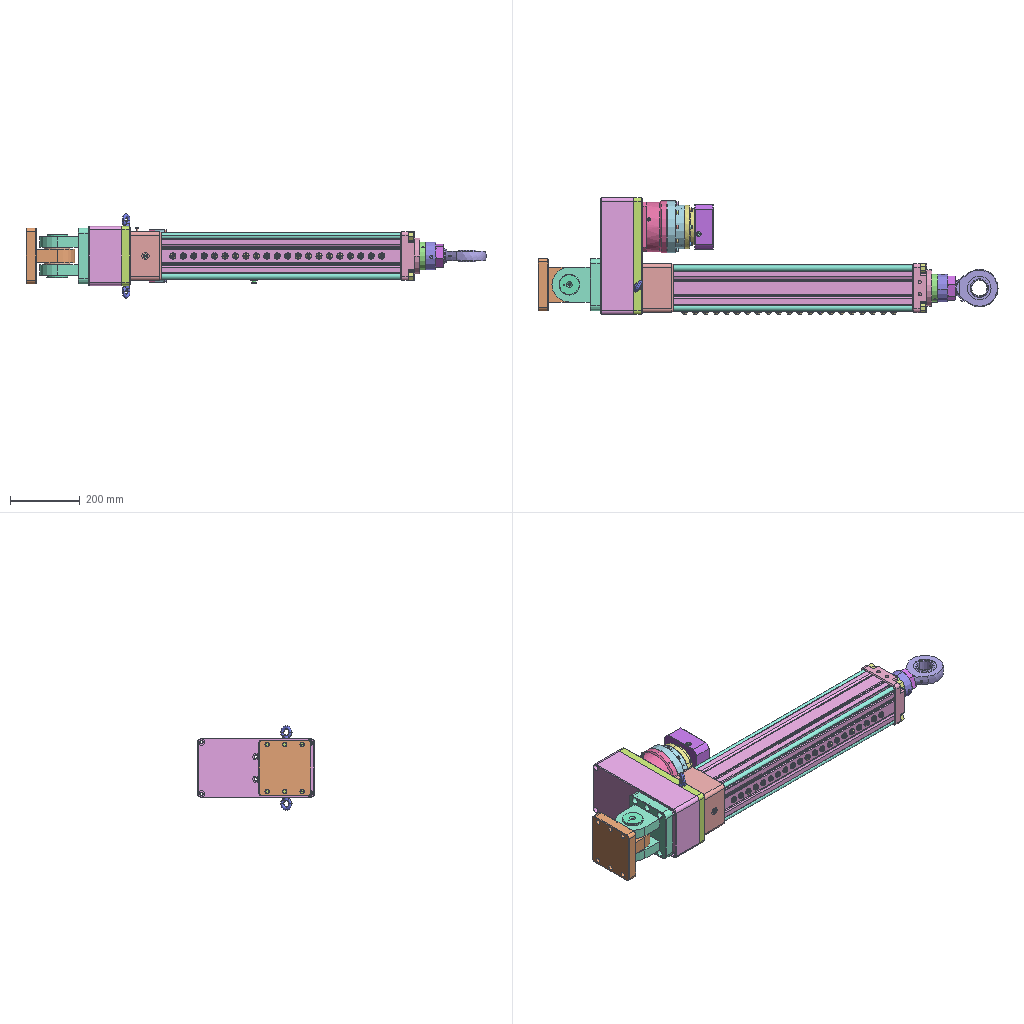Assembly | SolidWorks | 37 different items | 88 placed | box 1322 x 335 x 242 mm
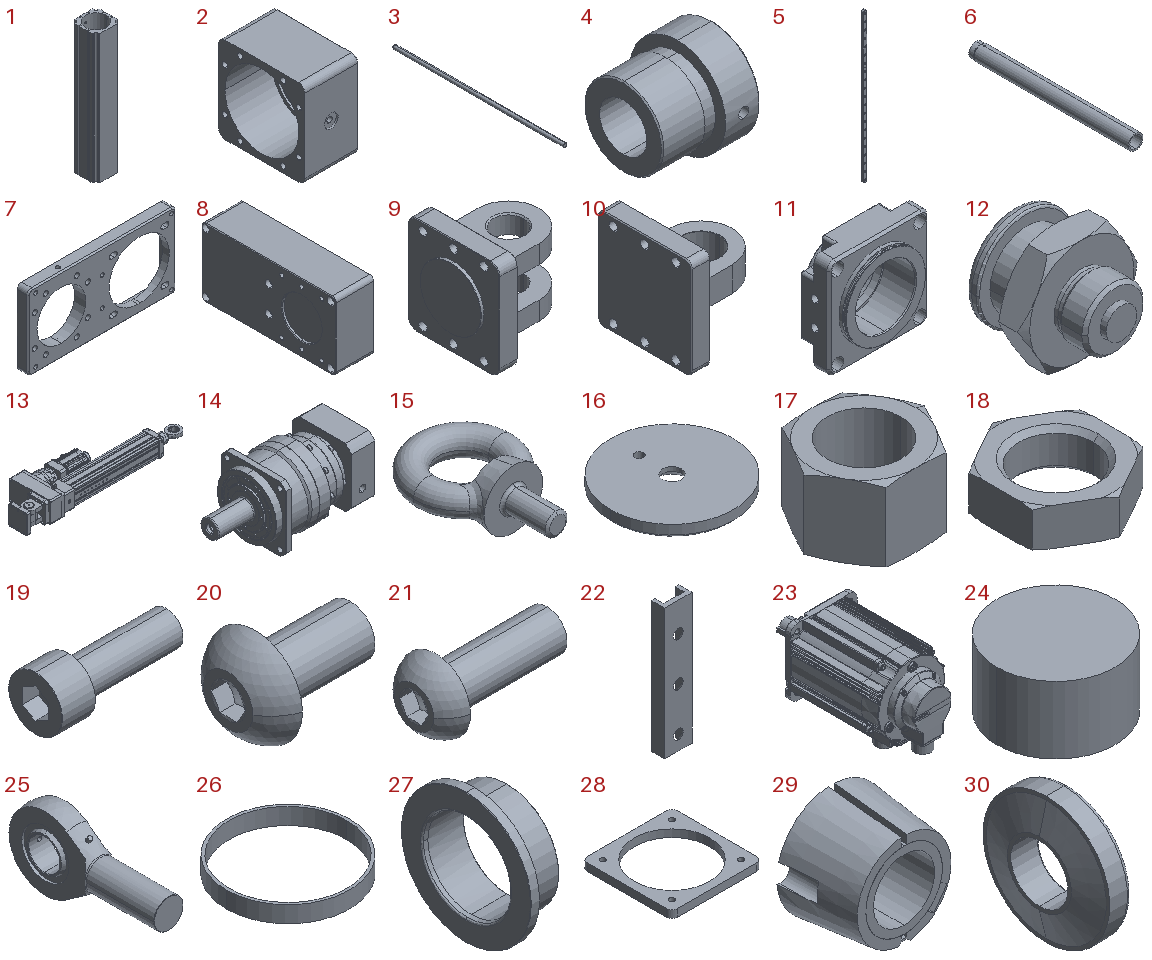Parts list (item | quantity | size | volume | features):
1 | x1 | 134 x 134 x 689 mm | 4449218 mm3 | features ICE 6, HoleWzd 5, Chamfer 3, CirPattern 3, Fillet 3, LPattern 2, MirrorPattern 2, Extrusion 1, MoveFace 1
2 | x1 | 98 x 140 x 140 mm | 787402 mm3 | features ICE 13, HoleWzd 7, Chamfer 4, MirrorPattern 4, CirPattern 1, Extrusion 1, Fillet 1
3 | x4 | 16 x 759 x 16 mm | 152408 mm3 | features Chamfer 1, Extrusion 1
4 | x1 | 74 x 79 x 79 mm | 198251 mm3 | features ICE 9, Chamfer 7, Draft 2, HoleWzd 2, Extrusion 1, Fillet 1, MirrorPattern 1, MoveFace 1
5 | x1 | 14 x 9 x 620 mm | 64305 mm3 | features ICE 2, Extrusion 1, Fillet 1, HoleWzd 1, LPattern 1
6 | x1 | 80 x 864.5 x 80 mm | 1857047 mm3 | features ICE 5, Chamfer 2, Extrusion 1, HoleWzd 1
7 | x1 | 335 x 25 x 170 mm | 717401 mm3 | features HoleWzd 9, ICE 4, MoveFace 4, MirrorPattern 3, Chamfer 1, Extrusion 1, Fillet 1
8 | x1 | 95 x 335 x 170 mm | 1808811 mm3 | features HoleWzd 3, MirrorPattern 3, Chamfer 2, Fillet 2, ICE 2, Extrusion 1
9 | x1 | 145 x 150 x 160 mm | 1190904 mm3 | features Chamfer 4, ICE 3, Fillet 2, Extrusion 1, HoleWzd 1, MirrorPattern 1
10 | x1 | 140 x 150 x 160 mm | 960906 mm3 | features Chamfer 4, ICE 3, Fillet 2, Extrusion 1, HoleWzd 1, MirrorPattern 1
11 | x1 | 140 x 65 x 140 mm | 538697 mm3 | features ICE 12, HoleWzd 11, Chamfer 7, Fillet 4, CirPattern 3, Extrusion 1, MirrorPattern 1, MoveFace 1, RevCut 1
12 | x1 | 19.63 x 18 x 17 mm | 2444 mm3 | features ICE 3, Revolution 2
13 | x1 | - | - | features BaseBody 82, RefSurface 62
14 | x1 | 300 x 150 x 150 mm | 3045756 mm3 | features BaseBody 51
15 | x2 | 36.2 x 52.1 x 21.1 mm | 7704 mm3 | features Fillet 2, Extrusion 1, LPattern 1, RevCut 1, Revolution 1, Sweep 1
16 | x2 | 60 x 60 x 6 mm | 15998 mm3 | features BaseBody 1
17 | x4 | 26.17 x 22.664 x 15.9 mm | 3864 mm3 | features Cut 2, Chamfer 1, Extrusion 1
18 | x1 | 61.887 x 71.299 x 21 mm | 39180 mm3 | features Cut 2, Chamfer 1, Extrusion 1
19 | x1 | 40 x 16 x 16 mm | 4081 mm3 | features BlendCut 1, Cut 1, Fillet 1, LPattern 1, RevCut 1, Revolution 1
20 | x1 | 12.75 x 9.5 x 9.5 mm | 314.028 mm3 | features RevCut 2, Revolution 2, Cut 1, LPattern 1, RefAxis 1
21 | x21 | 27.4 x 14 x 14 mm | 1571 mm3 | features RevCut 2, Revolution 2, Cut 1, LPattern 1, RefAxis 1
22 | x1 | 19 x 9 x 90 mm | 7114 mm3 | features Chamfer 1, Extrusion 1, HoleWzd 1, LPattern 1
23 | x1 | - | - | features RefSurface 59
24 | x2 | 8.8 x 8.8 x 5 mm | 304.106 mm3 | features Extrusion 1
25 | x1 | 42 x 217 x 108 mm | 356904 mm3 | features BaseBody 1
26 | x1 | 112 x 112 x 15 mm | 12900 mm3 | features Extrusion 1
27 | x2 | 24 x 75 x 75 mm | 28495 mm3 | features BaseBody 1, Chamfer 1, ICE 1
28 | x1 | 120 x 120 x 10 mm | 63169 mm3 | features HoleWzd 2, Extrusion 1, Fillet 1, ICE 1
29 | x1 | 56.795 x 38 x 56.678 mm | 48343 mm3 | features BaseBody 1, ICE 1
30 | x21 | 4 x 18 x 18 mm | 691.632 mm3 | features BaseBody 1
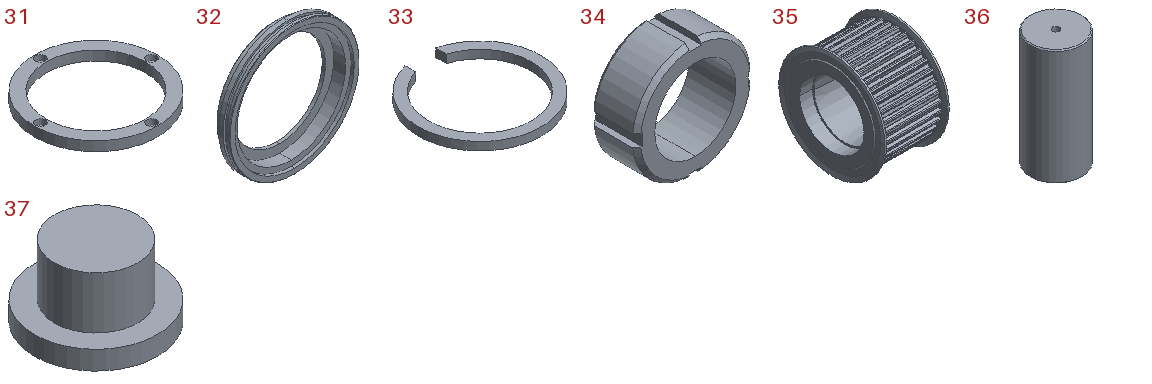31 | x1 | 103 x 103 x 8 mm | 22232 mm3 | features CirPattern 1, Extrusion 1, HoleWzd 1
32 | x1 | 120 x 17 x 120 mm | 45523 mm3 | features ICE 5, Chamfer 2, Extrusion 1
33 | x1 | 120 x 118.095 x 8 mm | 25215 mm3 | features Extrusion 1, ICE 1
34 | x1 | 57.689 x 23 x 57.689 mm | 29622 mm3 | features Chamfer 1, CirPattern 1, Extrusion 1, ICE 1
35 | x2 | 60 x 99 x 99 mm | 224539 mm3 | features ICE 4, Revolution 2, Chamfer 1, CirPattern 1, MirrorPattern 1
36 | x1 | 50 x 50 x 112 mm | 218046 mm3 | features HoleWzd 2, Chamfer 1, Extrusion 1
37 | x1 | 13 x 13 x 7.5 mm | 544.556 mm3 | features ICE 2, Extrusion 1
Mates (type | each side: item.copy, entity, surface, feature):
Coincident | 2.1 plane | assembly plane | 2 times
Concentric | assembly face | 34.1 face cylinder Boss-Extrude1
Concentric | 2.1 face cylinder Cut-Extrude1 | 32.1 face cylinder Boss-Extrude1
Concentric | assembly face | assembly face | 5 times
Coincident | 2.1 face plane Boss-Extrude1 | 1.1 face plane Boss-Extrude1
Coincident | assembly face | assembly face | 5 times
Concentric | assembly face | 19.1 face cylinder Base-Revolve
Coincident | assembly face | 19.1 face plane Base-Revolve
Tangent | 1.1 face cylinder Boss-Extrude1 | 5.1 face plane Boss-Extrude1
Concentric | 1.1 face cylinder Ø9.0 (9) Diameter Hole1 | 5.1 face cylinder M8 Tapped Hole1
Coincident | 2.1 face plane Cut-Extrude9 | 31.1 face plane Boss-Extrude1
Concentric | 2.1 face cylinder Cut-Extrude9 | 31.1 face cylinder Boss-Extrude1
Concentric | 3.1 face cylinder Boss-Extrude1 | 17.1 face cylinder Base-Extrude
Concentric | assembly face | 18.1 face cylinder Base-Extrude
DistanceDim | assembly face | 18.1 face plane Base-Extrude
Concentric | 3.1 face cylinder Boss-Extrude1 | assembly face
Coincident | 1.1 face plane Boss-Extrude1 | assembly face
Concentric | 3.2 face cylinder Boss-Extrude1 | assembly face
Coincident | 3.1 face plane Boss-Extrude1 | 3.2 face plane Boss-Extrude1
Concentric | 3.3 face cylinder Boss-Extrude1 | assembly face
Coincident | 3.3 face plane Boss-Extrude1 | assembly face
Concentric | 3.4 face cylinder Boss-Extrude1 | assembly face
Coincident | 3.4 face plane Boss-Extrude1 | assembly face
Parallel | 18.1 face plane Base-Extrude | assembly face
Parallel | assembly face | assembly face
Coincident | 17.1 face plane Base-Extrude | assembly face
Parallel | 33.1 face plane Cut-Extrude1 | assembly face
Concentric | 2.1 face cylinder G1/8 Tapped Hole1 | 37.1 face cylinder Cut-Extrude1
Coincident | assembly face | 20.1 face plane Revolve1
Concentric | 29.1 face | 35.1 face cone Cut-Extrude4
Coincident | 29.1 face plane Input1 | 35.1 face plane Cut-Extrude3
Coincident | assembly face | 35.1 face plane Revolve1
Coincident | assembly face | 35.2 face plane Revolve1
Coincident | 1.1 face plane Boss-Extrude1 | 30.1 face plane Input1
Concentric | 1.1 face cylinder Ø9.0 (9) Diameter Hole1 | 30.1 face cylinder Input1
Concentric | 1.1 face cylinder LPattern1 | 5.1 face cylinder LPattern1
DistanceDim | assembly face | assembly face | 2 times
Concentric | 1.1 face cylinder G1/8 Tapped Hole1 | 12.1 face cylinder Revolve1
Coincident | 1.1 face plane Boss-Extrude1 | 12.1 face plane Revolve1
Concentric | 1.1 face cylinder G1/8 Tapped Hole2 | 24.1 face cylinder Boss-Extrude1
Coincident | 1.1 face plane Boss-Extrude1 | 24.1 face plane Boss-Extrude1
Concentric | 1.1 face cylinder G1/8 Tapped Hole2 | 24.2 face cylinder Boss-Extrude1
Coincident | 1.1 face plane Boss-Extrude1 | 24.2 face plane Boss-Extrude1
Concentric | 21.1 face cylinder Revolve1 | 30.1 face cylinder Input1
Coincident | 21.1 face plane Revolve1 | 30.1 face plane Input1
Concentric | 22.1 face cone LPattern1 | assembly face
Concentric | assembly face | 29.1 face
Concentric | 32.1 face cylinder Boss-Extrude2 | 7.1 face cylinder Cut-Extrude1
Coincident | 2.1 face plane Boss-Extrude1 | 7.1 face plane Boss-Extrude1
Concentric | 7.1 edge | 8.1 edge
Coincident | 7.1 face plane Boss-Extrude1 | 8.1 face plane Boss-Extrude1
Parallel | 7.1 face plane Boss-Extrude1 | 8.1 face plane Boss-Extrude1
Coincident | 8.1 face plane Boss-Extrude1 | assembly face
Coincident | 8.1 face plane Boss-Extrude1 | 9.1 face plane Boss-Extrude1
Parallel | 8.1 face plane Boss-Extrude1 | 9.1 face plane Mirror1
Concentric | 8.1 face cylinder Cut-Extrude2 | 9.1 face cylinder Boss-Extrude3
Concentric | 9.1 face cylinder Mirror1 | 10.1 face cylinder Cut-Extrude1
Width | 9.1 face plane Mirror1 | 9.1 face plane Boss-Extrude2 | 10.1 face plane Boss-Extrude2 | 10.1 face plane Boss-Extrude2
DistanceDim | 3.1 face plane Boss-Extrude1 | 2.1 face plane Boss-Extrude1
Coincident | 28.1 face plane Boss-Extrude1 | 7.1 face plane Cut-Extrude3
Parallel | 28.1 face plane Boss-Extrude1 | 7.1 face plane Cut-Extrude3
Slot | 28.1 face cylinder Cut-Extrude1 | 7.1 face cylinder Cut-Extrude2
Concentric | 25.1 face cylinder Input1 | assembly face | 2 times
Concentric | 18.1 face cylinder Base-Extrude | 25.1 face cylinder Input1
Coincident | 18.1 face plane Base-Extrude | assembly face | 2 times
Coincident | assembly face | 6.1 face plane Boss-Extrude1
Concentric | 28.1 edge | 29.1 face
Coincident | assembly face | 13.1 face plane 125 Front End Cover Non-flange-1-solid1 | 2 times
Concentric | 6.1 face cylinder Cut-Extrude4 | assembly face
Coincident | 6.1 face plane Boss-Extrude1 | assembly face
Parallel | assembly face | 25.1 face plane Input1
DistanceDim | 18.1 face plane Base-Extrude | 25.1 face plane Input1
Parallel | 2.1 face plane Boss-Extrude1 | 1.1 face plane Boss-Extrude1
Concentric | 2.1 face cylinder M16 Tapped Hole1 | 3.1 face cylinder Boss-Extrude1
Parallel | 2.1 face plane Boss-Extrude1 | 8.1 face plane Boss-Extrude1
Concentric | 15.1 face cylinder Base-Extrude | 7.1 face cylinder Mirror2
Coincident | 15.1 face plane Boss-Revolve1 | 7.1 face plane Boss-Extrude1
Concentric | 23.1 face cylinder Surface-Input22 | 14.1 face cylinder Stage 1 Integral Sun Gear with Jacket Outline KB115-D28SLDPRT-1-solid2
Coincident | 23.1 face plane Surface-Input2 | 14.1 face plane Motor Flange AKB115 D110-M8-145F130H52-1-solid1
Parallel | 23.1 face plane Surface-Input31 | 14.1 face plane Motor Flange AKB115 D110-M8-145F130H52-1-solid1
Slot | 14.1 face cylinder Stage 1 Ring Gear with Output Shaft KS142 Outline-1-solid1 | 7.1 face cylinder Cut-Extrude2
Parallel | 7.1 face plane Boss-Extrude1 | 14.1 face plane Stage 1 Ring Gear with Output Shaft KS142 Outline-1-solid1
Coincident | 7.1 face plane Boss-Extrude1 | 14.1 face plane Stage 1 Ring Gear with Output Shaft KS142 Outline-1-solid1
LimitDistanceDim | assembly face | assembly face
Concentric | 6.1 face cylinder Cut-Extrude4 | 4.1 face cylinder Cut-Extrude3
Coincident | 6.1 face plane Boss-Extrude1 | 4.1 face plane Cut-Extrude3
Coincident | 18.1 face plane Base-Extrude | 4.1 face plane Cut-Extrude1
Concentric | 25.1 face cylinder Input1 | 4.1 face cylinder M42x3.0 Tapped Hole1
Concentric | 9.1 face cylinder Mirror1 | 16.1 face cylinder Input1
Concentric | 9.1 face cylinder Cut-Extrude1 | 27.1 face cylinder Input1
Concentric | 9.1 face cylinder Cut-Extrude1 | 16.2 edge
Coincident | 9.1 face plane Boss-Extrude2 | 27.1 face plane Input1
Concentric | 9.1 face cylinder Mirror1 | 27.2 face cylinder Input1
Coincident | 9.1 face plane Mirror1 | 27.2 face plane Input1
LimitDistanceDim | 4.1 face plane Cut-Extrude1 | assembly face
Parallel | 8.1 face plane Boss-Extrude1 | 10.1 face plane Boss-Extrude1
Concentric | 9.1 face cylinder Mirror1 | 36.1 face cylinder Boss-Extrude1
Width | 36.1 face plane Boss-Extrude1 | 36.1 face plane Boss-Extrude1 | 9.1 face plane Mirror1 | 9.1 face plane Boss-Extrude2
Coincident | 16.1 face plane Input1 | 36.1 face plane Boss-Extrude1
Coincident | 16.2 face plane Input1 | 36.1 face plane Boss-Extrude1
Concentric | 14.1 face cylinder Stage 1 Ring Gear with Output Shaft KS142 Outline-1-solid1 | assembly face
Coincident | 14.1 face plane Stage 1 Ring Gear with Output Shaft KS142 Outline-1-solid1 | assembly face
Coincident | 29.1 face plane Input1 | assembly face
Parallel | 1.1 face plane Boss-Extrude1 | 11.1 face plane Cut-Extrude15
Coincident | 1.1 face plane Boss-Extrude1 | 11.1 face plane Boss-Extrude1
DistanceDim | 25.1 face cylinder Input1 | 11.1 face plane Boss-Extrude1